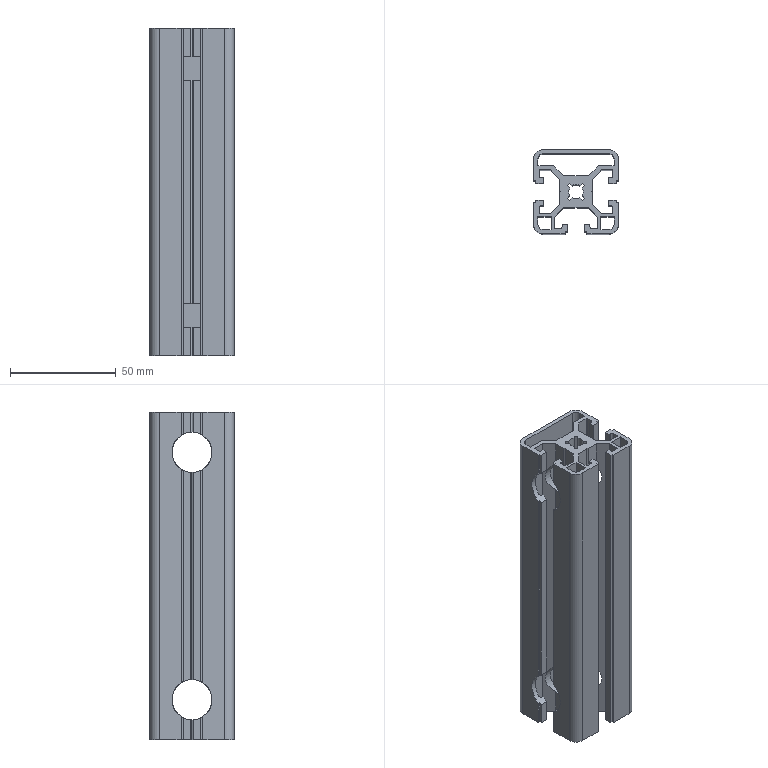Part | SolidWorks | features BaseBody 1, HoleWzd 1, MoveFace 1 | 1 solid | 242 faces | box 40 x 40 x 155 mm | volume 83386 mm3 | plane 187 | cylinder 55 | commonest cylinder face diameters 6.8 x15 2 x14 19 x12 1 x6 5 x4 9 x4